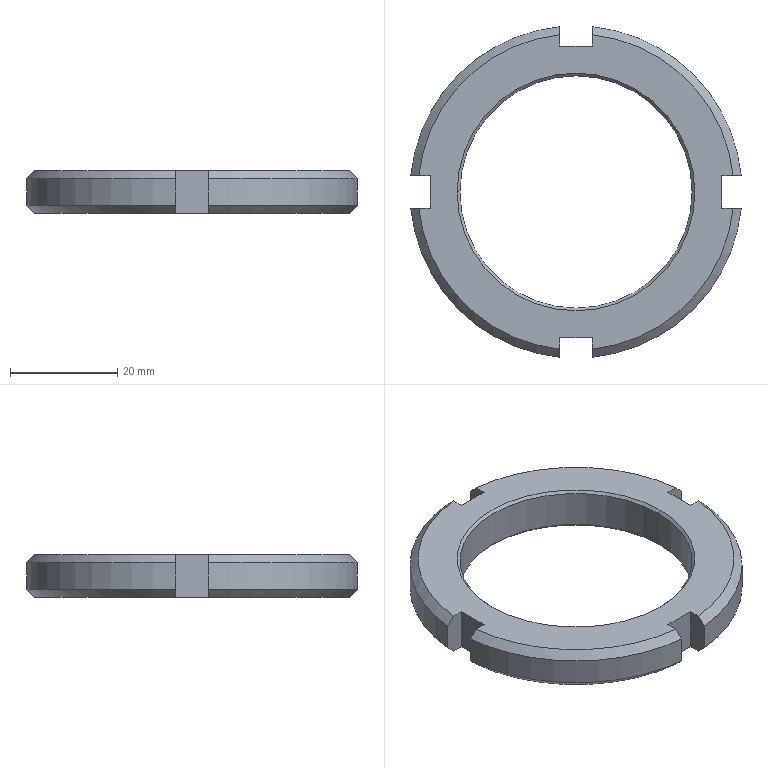Part | SolidWorks | features BaseBody 1 | 1 solid | 32 faces | box 61.709 x 61.709 x 8 mm | volume 11209 mm3 | plane 14 | cone 12 | cylinder 6 | commonest cylinder face diameters 62 x4 43.376 x2
STEP:
#1=CARTESIAN_POINT('',(-21.688,0.,7.5));
#2=VERTEX_POINT('',#1);
#3=CARTESIAN_POINT('',(21.688,0.,7.5));
#4=VERTEX_POINT('',#3);
#5=CARTESIAN_POINT('',(0.,0.,7.5));
#6=DIRECTION('',(0.,0.,1.));
#7=DIRECTION('',(1.,0.,0.));
#8=AXIS2_PLACEMENT_3D('',#5,#6,#7);
#9=CIRCLE('',#8,21.688);
#10=EDGE_CURVE('',#2,#4,#9,.T.);
#11=ORIENTED_EDGE('',*,*,#10,.F.);
#12=CARTESIAN_POINT('',(-22.188,0.,8.));
#13=VERTEX_POINT('',#12);
#14=CARTESIAN_POINT('',(-21.688,0.,7.5));
#15=DIRECTION('',(-0.7071,0.,0.7071));
#16=VECTOR('',#15,1000.);
#17=LINE('',#14,#16);
#18=EDGE_CURVE('',#2,#13,#17,.T.);
#19=ORIENTED_EDGE('',*,*,#18,.T.);
#20=CARTESIAN_POINT('',(22.188,0.,8.));
#21=VERTEX_POINT('',#20);
#22=CARTESIAN_POINT('',(0.,0.,8.));
#23=DIRECTION('',(0.,0.,-1.));
#24=DIRECTION('',(1.,0.,0.));
#25=AXIS2_PLACEMENT_3D('',#22,#23,#24);
#26=CIRCLE('',#25,22.188);
#27=EDGE_CURVE('',#21,#13,#26,.T.);
#28=ORIENTED_EDGE('',*,*,#27,.F.);
#29=CARTESIAN_POINT('',(21.688,0.,7.5));
#30=DIRECTION('',(0.7071,0.,0.7071));
#31=VECTOR('',#30,1000.);
#32=LINE('',#29,#31);
#33=EDGE_CURVE('',#4,#21,#32,.T.);
#34=ORIENTED_EDGE('',*,*,#33,.F.);
#35=EDGE_LOOP('',(#11,#19,#28,#34));
#36=FACE_OUTER_BOUND('',#35,.T.);
#37=CARTESIAN_POINT('',(0.,0.,7.5));
#38=DIRECTION('',(0.,0.,1.));
#39=DIRECTION('',(1.,0.,0.));
#40=AXIS2_PLACEMENT_3D('',#37,#38,#39);
#41=CONICAL_SURFACE('',#40,21.688,0.7854);
#42=ADVANCED_FACE('',(#36),#41,.F.);
#43=CARTESIAN_POINT('',(21.688,0.,0.5));
#44=VERTEX_POINT('',#43);
#45=CARTESIAN_POINT('',(-21.688,0.,0.5));
#46=VERTEX_POINT('',#45);
#47=CARTESIAN_POINT('',(0.,0.,0.5));
#48=DIRECTION('',(0.,0.,-1.));
#49=DIRECTION('',(1.,0.,0.));
#50=AXIS2_PLACEMENT_3D('',#47,#48,#49);
#51=CIRCLE('',#50,21.688);
#52=EDGE_CURVE('',#44,#46,#51,.T.);
#53=ORIENTED_EDGE('',*,*,#52,.F.);
#54=CARTESIAN_POINT('',(22.188,0.,0.));
#55=VERTEX_POINT('',#54);
#56=CARTESIAN_POINT('',(22.188,0.,0.));
#57=DIRECTION('',(0.7071,0.,-0.7071));
#58=VECTOR('',#57,1000.);
#59=LINE('',#56,#58);
#60=EDGE_CURVE('',#44,#55,#59,.T.);
#61=ORIENTED_EDGE('',*,*,#60,.T.);
#62=CARTESIAN_POINT('',(-22.188,0.,0.));
#63=VERTEX_POINT('',#62);
#64=CARTESIAN_POINT('',(0.,0.,0.));
#65=DIRECTION('',(0.,0.,1.));
#66=DIRECTION('',(1.,0.,0.));
#67=AXIS2_PLACEMENT_3D('',#64,#65,#66);
#68=CIRCLE('',#67,22.188);
#69=EDGE_CURVE('',#63,#55,#68,.T.);
#70=ORIENTED_EDGE('',*,*,#69,.F.);
#71=CARTESIAN_POINT('',(-22.188,0.,0.));
#72=DIRECTION('',(-0.7071,0.,-0.7071));
#73=VECTOR('',#72,1000.);
#74=LINE('',#71,#73);
#75=EDGE_CURVE('',#46,#63,#74,.T.);
#76=ORIENTED_EDGE('',*,*,#75,.F.);
#77=EDGE_LOOP('',(#53,#61,#70,#76));
#78=FACE_OUTER_BOUND('',#77,.T.);
#79=CARTESIAN_POINT('',(0.,0.,0.));
#80=DIRECTION('',(0.,0.,-1.));
#81=DIRECTION('',(-1.,0.,0.));
#82=AXIS2_PLACEMENT_3D('',#79,#80,#81);
#83=CONICAL_SURFACE('',#82,22.188,0.7854);
#84=ADVANCED_FACE('',(#78),#83,.F.);
#85=ORIENTED_EDGE('',*,*,#10,.T.);
#86=CARTESIAN_POINT('',(21.688,0.,8.));
#87=DIRECTION('',(0.,0.,-1.));
#88=VECTOR('',#87,1000.);
#89=LINE('',#86,#88);
#90=EDGE_CURVE('',#4,#44,#89,.T.);
#91=ORIENTED_EDGE('',*,*,#90,.T.);
#92=ORIENTED_EDGE('',*,*,#52,.T.);
#93=CARTESIAN_POINT('',(-21.688,0.,8.));
#94=DIRECTION('',(0.,0.,-1.));
#95=VECTOR('',#94,1000.);
#96=LINE('',#93,#95);
#97=EDGE_CURVE('',#2,#46,#96,.T.);
#98=ORIENTED_EDGE('',*,*,#97,.F.);
#99=EDGE_LOOP('',(#85,#91,#92,#98));
#100=FACE_OUTER_BOUND('',#99,.T.);
#101=CARTESIAN_POINT('',(0.,0.,8.));
#102=DIRECTION('',(0.,0.,-1.));
#103=DIRECTION('',(-1.,0.,0.));
#104=AXIS2_PLACEMENT_3D('',#101,#102,#103);
#105=CYLINDRICAL_SURFACE('',#104,21.688);
#106=ADVANCED_FACE('',(#100),#105,.F.);
#107=CARTESIAN_POINT('',(3.,30.854,6.5));
#108=VERTEX_POINT('',#107);
#109=CARTESIAN_POINT('',(30.854,3.,6.5));
#110=VERTEX_POINT('',#109);
#111=CARTESIAN_POINT('',(0.,0.,6.5));
#112=DIRECTION('',(0.,0.,-1.));
#113=DIRECTION('',(1.,0.,0.));
#114=AXIS2_PLACEMENT_3D('',#111,#112,#113);
#115=CIRCLE('',#114,31.);
#116=EDGE_CURVE('',#108,#110,#115,.T.);
#117=ORIENTED_EDGE('',*,*,#116,.T.);
#118=CARTESIAN_POINT('',(30.854,3.,1.5));
#119=VERTEX_POINT('',#118);
#120=CARTESIAN_POINT('',(30.854,3.,0.));
#121=DIRECTION('',(0.,0.,1.));
#122=VECTOR('',#121,1000.);
#123=LINE('',#120,#122);
#124=EDGE_CURVE('',#119,#110,#123,.T.);
#125=ORIENTED_EDGE('',*,*,#124,.F.);
#126=CARTESIAN_POINT('',(3.,30.854,1.5));
#127=VERTEX_POINT('',#126);
#128=CARTESIAN_POINT('',(0.,0.,1.5));
#129=DIRECTION('',(0.,0.,1.));
#130=DIRECTION('',(1.,0.,0.));
#131=AXIS2_PLACEMENT_3D('',#128,#129,#130);
#132=CIRCLE('',#131,31.);
#133=EDGE_CURVE('',#119,#127,#132,.T.);
#134=ORIENTED_EDGE('',*,*,#133,.T.);
#135=CARTESIAN_POINT('',(3.,30.854,0.));
#136=DIRECTION('',(0.,0.,1.));
#137=VECTOR('',#136,1000.);
#138=LINE('',#135,#137);
#139=EDGE_CURVE('',#127,#108,#138,.T.);
#140=ORIENTED_EDGE('',*,*,#139,.T.);
#141=EDGE_LOOP('',(#117,#125,#134,#140));
#142=FACE_OUTER_BOUND('',#141,.T.);
#143=CARTESIAN_POINT('',(0.,0.,8.));
#144=DIRECTION('',(0.,0.,-1.));
#145=DIRECTION('',(-1.,0.,0.));
#146=AXIS2_PLACEMENT_3D('',#143,#144,#145);
#147=CYLINDRICAL_SURFACE('',#146,31.);
#148=ADVANCED_FACE('',(#142),#147,.T.);
#149=CARTESIAN_POINT('',(29.347,3.,8.));
#150=VERTEX_POINT('',#149);
#151=CARTESIAN_POINT('',(30.854,3.,6.5));
#152=CARTESIAN_POINT('',(30.441,3.,6.912));
#153=CARTESIAN_POINT('',(30.027,3.,7.323));
#154=CARTESIAN_POINT('',(29.614,3.,7.735));
#155=CARTESIAN_POINT('',(29.525,3.,7.823));
#156=CARTESIAN_POINT('',(29.436,3.,7.912));
#157=CARTESIAN_POINT('',(29.347,3.,8.));
#158=B_SPLINE_CURVE_WITH_KNOTS('',3,(#151,#152,#153,#154,#155,#156,#157),.UNSPECIFIED.,.F.,.F.,(4,3,4),(0.006071,0.007821,0.008198),.UNSPECIFIED.);
#159=EDGE_CURVE('',#110,#150,#158,.T.);
#160=ORIENTED_EDGE('',*,*,#159,.F.);
#161=ORIENTED_EDGE('',*,*,#116,.F.);
#162=CARTESIAN_POINT('',(3.,29.347,8.));
#163=VERTEX_POINT('',#162);
#164=CARTESIAN_POINT('',(3.,29.347,8.));
#165=CARTESIAN_POINT('',(3.,29.436,7.912));
#166=CARTESIAN_POINT('',(3.,29.525,7.823));
#167=CARTESIAN_POINT('',(3.,29.614,7.735));
#168=CARTESIAN_POINT('',(3.,30.027,7.323));
#169=CARTESIAN_POINT('',(3.,30.441,6.912));
#170=CARTESIAN_POINT('',(3.,30.854,6.5));
#171=B_SPLINE_CURVE_WITH_KNOTS('',3,(#164,#165,#166,#167,#168,#169,#170),.UNSPECIFIED.,.F.,.F.,(4,3,4),(0.007445,0.007821,0.009572),.UNSPECIFIED.);
#172=EDGE_CURVE('',#163,#108,#171,.T.);
#173=ORIENTED_EDGE('',*,*,#172,.F.);
#174=CARTESIAN_POINT('',(0.,0.,8.));
#175=DIRECTION('',(0.,0.,1.));
#176=DIRECTION('',(1.,0.,0.));
#177=AXIS2_PLACEMENT_3D('',#174,#175,#176);
#178=CIRCLE('',#177,29.5);
#179=EDGE_CURVE('',#150,#163,#178,.T.);
#180=ORIENTED_EDGE('',*,*,#179,.F.);
#181=EDGE_LOOP('',(#160,#161,#173,#180));
#182=FACE_OUTER_BOUND('',#181,.T.);
#183=CARTESIAN_POINT('',(0.,0.,8.));
#184=DIRECTION('',(0.,0.,-1.));
#185=DIRECTION('',(-1.,0.,0.));
#186=AXIS2_PLACEMENT_3D('',#183,#184,#185);
#187=CONICAL_SURFACE('',#186,29.5,0.7854);
#188=ADVANCED_FACE('',(#182),#187,.T.);
#189=CARTESIAN_POINT('',(29.347,3.,0.));
#190=VERTEX_POINT('',#189);
#191=CARTESIAN_POINT('',(29.347,3.,0.));
#192=CARTESIAN_POINT('',(29.436,3.,0.08842));
#193=CARTESIAN_POINT('',(29.525,3.,0.1768));
#194=CARTESIAN_POINT('',(29.614,3.,0.2653));
#195=CARTESIAN_POINT('',(30.027,3.,0.6768));
#196=CARTESIAN_POINT('',(30.441,3.,1.088));
#197=CARTESIAN_POINT('',(30.854,3.,1.5));
#198=B_SPLINE_CURVE_WITH_KNOTS('',3,(#191,#192,#193,#194,#195,#196,#197),.UNSPECIFIED.,.F.,.F.,(4,3,4),(0.007445,0.007821,0.009572),.UNSPECIFIED.);
#199=EDGE_CURVE('',#190,#119,#198,.T.);
#200=ORIENTED_EDGE('',*,*,#199,.F.);
#201=CARTESIAN_POINT('',(3.,29.347,0.));
#202=VERTEX_POINT('',#201);
#203=CARTESIAN_POINT('',(0.,0.,0.));
#204=DIRECTION('',(0.,0.,-1.));
#205=DIRECTION('',(1.,0.,0.));
#206=AXIS2_PLACEMENT_3D('',#203,#204,#205);
#207=CIRCLE('',#206,29.5);
#208=EDGE_CURVE('',#202,#190,#207,.T.);
#209=ORIENTED_EDGE('',*,*,#208,.F.);
#210=CARTESIAN_POINT('',(3.,30.854,1.5));
#211=CARTESIAN_POINT('',(3.,30.441,1.088));
#212=CARTESIAN_POINT('',(3.,30.027,0.6768));
#213=CARTESIAN_POINT('',(3.,29.614,0.2653));
#214=CARTESIAN_POINT('',(3.,29.525,0.1768));
#215=CARTESIAN_POINT('',(3.,29.436,0.08842));
#216=CARTESIAN_POINT('',(3.,29.347,0.));
#217=B_SPLINE_CURVE_WITH_KNOTS('',3,(#210,#211,#212,#213,#214,#215,#216),.UNSPECIFIED.,.F.,.F.,(4,3,4),(0.006071,0.007821,0.008198),.UNSPECIFIED.);
#218=EDGE_CURVE('',#127,#202,#217,.T.);
#219=ORIENTED_EDGE('',*,*,#218,.F.);
#220=ORIENTED_EDGE('',*,*,#133,.F.);
#221=EDGE_LOOP('',(#200,#209,#219,#220));
#222=FACE_OUTER_BOUND('',#221,.T.);
#223=CARTESIAN_POINT('',(0.,0.,1.5));
#224=DIRECTION('',(0.,0.,1.));
#225=DIRECTION('',(1.,0.,0.));
#226=AXIS2_PLACEMENT_3D('',#223,#224,#225);
#227=CONICAL_SURFACE('',#226,31.,0.7854);
#228=ADVANCED_FACE('',(#222),#227,.T.);
#229=CARTESIAN_POINT('',(-30.854,3.,6.5));
#230=VERTEX_POINT('',#229);
#231=CARTESIAN_POINT('',(-3.,30.854,6.5));
#232=VERTEX_POINT('',#231);
#233=CARTESIAN_POINT('',(0.,0.,6.5));
#234=DIRECTION('',(0.,0.,-1.));
#235=DIRECTION('',(1.,0.,0.));
#236=AXIS2_PLACEMENT_3D('',#233,#234,#235);
#237=CIRCLE('',#236,31.);
#238=EDGE_CURVE('',#230,#232,#237,.T.);
#239=ORIENTED_EDGE('',*,*,#238,.T.);
#240=CARTESIAN_POINT('',(-3.,30.854,1.5));
#241=VERTEX_POINT('',#240);
#242=CARTESIAN_POINT('',(-3.,30.854,0.));
#243=DIRECTION('',(0.,0.,1.));
#244=VECTOR('',#243,1000.);
#245=LINE('',#242,#244);
#246=EDGE_CURVE('',#241,#232,#245,.T.);
#247=ORIENTED_EDGE('',*,*,#246,.F.);
#248=CARTESIAN_POINT('',(-30.854,3.,1.5));
#249=VERTEX_POINT('',#248);
#250=CARTESIAN_POINT('',(0.,0.,1.5));
#251=DIRECTION('',(0.,0.,1.));
#252=DIRECTION('',(1.,0.,0.));
#253=AXIS2_PLACEMENT_3D('',#250,#251,#252);
#254=CIRCLE('',#253,31.);
#255=EDGE_CURVE('',#241,#249,#254,.T.);
#256=ORIENTED_EDGE('',*,*,#255,.T.);
#257=CARTESIAN_POINT('',(-30.854,3.,0.));
#258=DIRECTION('',(0.,0.,1.));
#259=VECTOR('',#258,1000.);
#260=LINE('',#257,#259);
#261=EDGE_CURVE('',#249,#230,#260,.T.);
#262=ORIENTED_EDGE('',*,*,#261,.T.);
#263=EDGE_LOOP('',(#239,#247,#256,#262));
#264=FACE_OUTER_BOUND('',#263,.T.);
#265=CARTESIAN_POINT('',(0.,0.,8.));
#266=DIRECTION('',(0.,0.,-1.));
#267=DIRECTION('',(-1.,0.,0.));
#268=AXIS2_PLACEMENT_3D('',#265,#266,#267);
#269=CYLINDRICAL_SURFACE('',#268,31.);
#270=ADVANCED_FACE('',(#264),#269,.T.);
#271=CARTESIAN_POINT('',(-3.,29.347,8.));
#272=VERTEX_POINT('',#271);
#273=CARTESIAN_POINT('',(-3.,30.854,6.5));
#274=CARTESIAN_POINT('',(-3.,30.441,6.912));
#275=CARTESIAN_POINT('',(-3.,30.027,7.323));
#276=CARTESIAN_POINT('',(-3.,29.614,7.735));
#277=CARTESIAN_POINT('',(-3.,29.525,7.823));
#278=CARTESIAN_POINT('',(-3.,29.436,7.912));
#279=CARTESIAN_POINT('',(-3.,29.347,8.));
#280=B_SPLINE_CURVE_WITH_KNOTS('',3,(#273,#274,#275,#276,#277,#278,#279),.UNSPECIFIED.,.F.,.F.,(4,3,4),(0.006071,0.007821,0.008198),.UNSPECIFIED.);
#281=EDGE_CURVE('',#232,#272,#280,.T.);
#282=ORIENTED_EDGE('',*,*,#281,.F.);
#283=ORIENTED_EDGE('',*,*,#238,.F.);
#284=CARTESIAN_POINT('',(-29.347,3.,8.));
#285=VERTEX_POINT('',#284);
#286=CARTESIAN_POINT('',(-29.347,3.,8.));
#287=CARTESIAN_POINT('',(-29.712,3.,7.637));
#288=CARTESIAN_POINT('',(-30.076,3.,7.274));
#289=CARTESIAN_POINT('',(-30.441,3.,6.912));
#290=CARTESIAN_POINT('',(-30.579,3.,6.774));
#291=CARTESIAN_POINT('',(-30.717,3.,6.637));
#292=CARTESIAN_POINT('',(-30.854,3.,6.5));
#293=B_SPLINE_CURVE_WITH_KNOTS('',3,(#286,#287,#288,#289,#290,#291,#292),.UNSPECIFIED.,.F.,.F.,(4,3,4),(0.006278,0.007821,0.008405),.UNSPECIFIED.);
#294=EDGE_CURVE('',#285,#230,#293,.T.);
#295=ORIENTED_EDGE('',*,*,#294,.F.);
#296=CARTESIAN_POINT('',(0.,0.,8.));
#297=DIRECTION('',(0.,0.,1.));
#298=DIRECTION('',(1.,0.,0.));
#299=AXIS2_PLACEMENT_3D('',#296,#297,#298);
#300=CIRCLE('',#299,29.5);
#301=EDGE_CURVE('',#272,#285,#300,.T.);
#302=ORIENTED_EDGE('',*,*,#301,.F.);
#303=EDGE_LOOP('',(#282,#283,#295,#302));
#304=FACE_OUTER_BOUND('',#303,.T.);
#305=CARTESIAN_POINT('',(0.,0.,8.));
#306=DIRECTION('',(0.,0.,-1.));
#307=DIRECTION('',(-1.,0.,0.));
#308=AXIS2_PLACEMENT_3D('',#305,#306,#307);
#309=CONICAL_SURFACE('',#308,29.5,0.7854);
#310=ADVANCED_FACE('',(#304),#309,.T.);
#311=CARTESIAN_POINT('',(-3.,29.347,0.));
#312=VERTEX_POINT('',#311);
#313=CARTESIAN_POINT('',(-3.,29.347,0.));
#314=CARTESIAN_POINT('',(-3.,29.436,0.08842));
#315=CARTESIAN_POINT('',(-3.,29.525,0.1768));
#316=CARTESIAN_POINT('',(-3.,29.614,0.2653));
#317=CARTESIAN_POINT('',(-3.,30.027,0.6768));
#318=CARTESIAN_POINT('',(-3.,30.441,1.088));
#319=CARTESIAN_POINT('',(-3.,30.854,1.5));
#320=B_SPLINE_CURVE_WITH_KNOTS('',3,(#313,#314,#315,#316,#317,#318,#319),.UNSPECIFIED.,.F.,.F.,(4,3,4),(0.007445,0.007821,0.009572),.UNSPECIFIED.);
#321=EDGE_CURVE('',#312,#241,#320,.T.);
#322=ORIENTED_EDGE('',*,*,#321,.F.);
#323=CARTESIAN_POINT('',(-29.347,3.,0.));
#324=VERTEX_POINT('',#323);
#325=CARTESIAN_POINT('',(0.,0.,0.));
#326=DIRECTION('',(0.,0.,-1.));
#327=DIRECTION('',(1.,0.,0.));
#328=AXIS2_PLACEMENT_3D('',#325,#326,#327);
#329=CIRCLE('',#328,29.5);
#330=EDGE_CURVE('',#324,#312,#329,.T.);
#331=ORIENTED_EDGE('',*,*,#330,.F.);
#332=CARTESIAN_POINT('',(-30.854,3.,1.5));
#333=CARTESIAN_POINT('',(-30.592,3.,1.238));
#334=CARTESIAN_POINT('',(-30.329,3.,0.9768));
#335=CARTESIAN_POINT('',(-30.066,3.,0.7152));
#336=CARTESIAN_POINT('',(-29.826,3.,0.4768));
#337=CARTESIAN_POINT('',(-29.587,3.,0.2384));
#338=CARTESIAN_POINT('',(-29.347,3.,0.));
#339=B_SPLINE_CURVE_WITH_KNOTS('',3,(#332,#333,#334,#335,#336,#337,#338),.UNSPECIFIED.,.F.,.F.,(4,3,4),(0.006709,0.007821,0.008836),.UNSPECIFIED.);
#340=EDGE_CURVE('',#249,#324,#339,.T.);
#341=ORIENTED_EDGE('',*,*,#340,.F.);
#342=ORIENTED_EDGE('',*,*,#255,.F.);
#343=EDGE_LOOP('',(#322,#331,#341,#342));
#344=FACE_OUTER_BOUND('',#343,.T.);
#345=CARTESIAN_POINT('',(0.,0.,1.5));
#346=DIRECTION('',(0.,0.,1.));
#347=DIRECTION('',(1.,0.,0.));
#348=AXIS2_PLACEMENT_3D('',#345,#346,#347);
#349=CONICAL_SURFACE('',#348,31.,0.7854);
#350=ADVANCED_FACE('',(#344),#349,.T.);
#351=CARTESIAN_POINT('',(-3.,-30.854,6.5));
#352=VERTEX_POINT('',#351);
#353=CARTESIAN_POINT('',(-30.854,-3.,6.5));
#354=VERTEX_POINT('',#353);
#355=CARTESIAN_POINT('',(0.,0.,6.5));
#356=DIRECTION('',(0.,0.,-1.));
#357=DIRECTION('',(1.,0.,0.));
#358=AXIS2_PLACEMENT_3D('',#355,#356,#357);
#359=CIRCLE('',#358,31.);
#360=EDGE_CURVE('',#352,#354,#359,.T.);
#361=ORIENTED_EDGE('',*,*,#360,.T.);
#362=CARTESIAN_POINT('',(-30.854,-3.,1.5));
#363=VERTEX_POINT('',#362);
#364=CARTESIAN_POINT('',(-30.854,-3.,0.));
#365=DIRECTION('',(0.,0.,1.));
#366=VECTOR('',#365,1000.);
#367=LINE('',#364,#366);
#368=EDGE_CURVE('',#363,#354,#367,.T.);
#369=ORIENTED_EDGE('',*,*,#368,.F.);
#370=CARTESIAN_POINT('',(-3.,-30.854,1.5));
#371=VERTEX_POINT('',#370);
#372=CARTESIAN_POINT('',(0.,0.,1.5));
#373=DIRECTION('',(0.,0.,1.));
#374=DIRECTION('',(1.,0.,0.));
#375=AXIS2_PLACEMENT_3D('',#372,#373,#374);
#376=CIRCLE('',#375,31.);
#377=EDGE_CURVE('',#363,#371,#376,.T.);
#378=ORIENTED_EDGE('',*,*,#377,.T.);
#379=CARTESIAN_POINT('',(-3.,-30.854,0.));
#380=DIRECTION('',(0.,0.,1.));
#381=VECTOR('',#380,1000.);
#382=LINE('',#379,#381);
#383=EDGE_CURVE('',#371,#352,#382,.T.);
#384=ORIENTED_EDGE('',*,*,#383,.T.);
#385=EDGE_LOOP('',(#361,#369,#378,#384));
#386=FACE_OUTER_BOUND('',#385,.T.);
#387=CARTESIAN_POINT('',(0.,0.,8.));
#388=DIRECTION('',(0.,0.,-1.));
#389=DIRECTION('',(-1.,0.,0.));
#390=AXIS2_PLACEMENT_3D('',#387,#388,#389);
#391=CYLINDRICAL_SURFACE('',#390,31.);
#392=ADVANCED_FACE('',(#386),#391,.T.);
#393=CARTESIAN_POINT('',(-29.347,-3.,8.));
#394=VERTEX_POINT('',#393);
#395=CARTESIAN_POINT('',(-30.854,-3.,6.5));
#396=CARTESIAN_POINT('',(-30.717,-3.,6.637));
#397=CARTESIAN_POINT('',(-30.579,-3.,6.774));
#398=CARTESIAN_POINT('',(-30.441,-3.,6.912));
#399=CARTESIAN_POINT('',(-30.076,-3.,7.274));
#400=CARTESIAN_POINT('',(-29.712,-3.,7.637));
#401=CARTESIAN_POINT('',(-29.347,-3.,8.));
#402=B_SPLINE_CURVE_WITH_KNOTS('',3,(#395,#396,#397,#398,#399,#400,#401),.UNSPECIFIED.,.F.,.F.,(4,3,4),(0.007238,0.007821,0.009365),.UNSPECIFIED.);
#403=EDGE_CURVE('',#354,#394,#402,.T.);
#404=ORIENTED_EDGE('',*,*,#403,.F.);
#405=ORIENTED_EDGE('',*,*,#360,.F.);
#406=CARTESIAN_POINT('',(-3.,-29.347,8.));
#407=VERTEX_POINT('',#406);
#408=CARTESIAN_POINT('',(-3.,-29.347,8.));
#409=CARTESIAN_POINT('',(-3.,-29.85,7.5));
#410=CARTESIAN_POINT('',(-3.,-30.352,7.));
#411=CARTESIAN_POINT('',(-3.,-30.854,6.5));
#412=B_SPLINE_CURVE_WITH_KNOTS('',3,(#408,#409,#410,#411),.UNSPECIFIED.,.F.,.F.,(4,4),(0.,0.002127),.UNSPECIFIED.);
#413=EDGE_CURVE('',#407,#352,#412,.T.);
#414=ORIENTED_EDGE('',*,*,#413,.F.);
#415=CARTESIAN_POINT('',(0.,0.,8.));
#416=DIRECTION('',(0.,0.,1.));
#417=DIRECTION('',(1.,0.,0.));
#418=AXIS2_PLACEMENT_3D('',#415,#416,#417);
#419=CIRCLE('',#418,29.5);
#420=EDGE_CURVE('',#394,#407,#419,.T.);
#421=ORIENTED_EDGE('',*,*,#420,.F.);
#422=EDGE_LOOP('',(#404,#405,#414,#421));
#423=FACE_OUTER_BOUND('',#422,.T.);
#424=CARTESIAN_POINT('',(0.,0.,8.));
#425=DIRECTION('',(0.,0.,-1.));
#426=DIRECTION('',(-1.,0.,0.));
#427=AXIS2_PLACEMENT_3D('',#424,#425,#426);
#428=CONICAL_SURFACE('',#427,29.5,0.7854);
#429=ADVANCED_FACE('',(#423),#428,.T.);
#430=CARTESIAN_POINT('',(-29.347,-3.,0.));
#431=VERTEX_POINT('',#430);
#432=CARTESIAN_POINT('',(-29.347,-3.,0.));
#433=CARTESIAN_POINT('',(-29.587,-3.,0.2384));
#434=CARTESIAN_POINT('',(-29.826,-3.,0.4768));
#435=CARTESIAN_POINT('',(-30.066,-3.,0.7152));
#436=CARTESIAN_POINT('',(-30.329,-3.,0.9768));
#437=CARTESIAN_POINT('',(-30.592,-3.,1.238));
#438=CARTESIAN_POINT('',(-30.854,-3.,1.5));
#439=B_SPLINE_CURVE_WITH_KNOTS('',3,(#432,#433,#434,#435,#436,#437,#438),.UNSPECIFIED.,.F.,.F.,(4,3,4),(0.006807,0.007821,0.008934),.UNSPECIFIED.);
#440=EDGE_CURVE('',#431,#363,#439,.T.);
#441=ORIENTED_EDGE('',*,*,#440,.F.);
#442=CARTESIAN_POINT('',(-3.,-29.347,0.));
#443=VERTEX_POINT('',#442);
#444=CARTESIAN_POINT('',(0.,0.,0.));
#445=DIRECTION('',(0.,0.,-1.));
#446=DIRECTION('',(1.,0.,0.));
#447=AXIS2_PLACEMENT_3D('',#444,#445,#446);
#448=CIRCLE('',#447,29.5);
#449=EDGE_CURVE('',#443,#431,#448,.T.);
#450=ORIENTED_EDGE('',*,*,#449,.F.);
#451=CARTESIAN_POINT('',(-3.,-30.854,1.5));
#452=CARTESIAN_POINT('',(-3.,-30.352,0.9999));
#453=CARTESIAN_POINT('',(-3.,-29.85,0.4999));
#454=CARTESIAN_POINT('',(-3.,-29.347,0.));
#455=B_SPLINE_CURVE_WITH_KNOTS('',3,(#451,#452,#453,#454),.UNSPECIFIED.,.F.,.F.,(4,4),(0.,0.002127),.UNSPECIFIED.);
#456=EDGE_CURVE('',#371,#443,#455,.T.);
#457=ORIENTED_EDGE('',*,*,#456,.F.);
#458=ORIENTED_EDGE('',*,*,#377,.F.);
#459=EDGE_LOOP('',(#441,#450,#457,#458));
#460=FACE_OUTER_BOUND('',#459,.T.);
#461=CARTESIAN_POINT('',(0.,0.,1.5));
#462=DIRECTION('',(0.,0.,1.));
#463=DIRECTION('',(1.,0.,0.));
#464=AXIS2_PLACEMENT_3D('',#461,#462,#463);
#465=CONICAL_SURFACE('',#464,31.,0.7854);
#466=ADVANCED_FACE('',(#460),#465,.T.);
#467=ORIENTED_EDGE('',*,*,#27,.T.);
#468=CARTESIAN_POINT('',(0.,0.,8.));
#469=DIRECTION('',(0.,0.,-1.));
#470=DIRECTION('',(1.,0.,0.));
#471=AXIS2_PLACEMENT_3D('',#468,#469,#470);
#472=CIRCLE('',#471,22.188);
#473=EDGE_CURVE('',#13,#21,#472,.T.);
#474=ORIENTED_EDGE('',*,*,#473,.T.);
#475=EDGE_LOOP('',(#467,#474));
#476=FACE_BOUND('',#475,.T.);
#477=CARTESIAN_POINT('',(27.254,3.,8.));
#478=VERTEX_POINT('',#477);
#479=CARTESIAN_POINT('',(27.254,3.,8.));
#480=DIRECTION('',(-1.,0.,0.));
#481=VECTOR('',#480,1000.);
#482=LINE('',#479,#481);
#483=EDGE_CURVE('',#150,#478,#482,.T.);
#484=ORIENTED_EDGE('',*,*,#483,.F.);
#485=ORIENTED_EDGE('',*,*,#179,.T.);
#486=CARTESIAN_POINT('',(3.,27.254,8.));
#487=VERTEX_POINT('',#486);
#488=CARTESIAN_POINT('',(3.,27.254,8.));
#489=DIRECTION('',(0.,1.,0.));
#490=VECTOR('',#489,1000.);
#491=LINE('',#488,#490);
#492=EDGE_CURVE('',#487,#163,#491,.T.);
#493=ORIENTED_EDGE('',*,*,#492,.F.);
#494=CARTESIAN_POINT('',(-3.,27.254,8.));
#495=VERTEX_POINT('',#494);
#496=CARTESIAN_POINT('',(3.,27.254,8.));
#497=DIRECTION('',(1.,0.,0.));
#498=VECTOR('',#497,1000.);
#499=LINE('',#496,#498);
#500=EDGE_CURVE('',#495,#487,#499,.T.);
#501=ORIENTED_EDGE('',*,*,#500,.F.);
#502=CARTESIAN_POINT('',(-3.,27.254,8.));
#503=DIRECTION('',(0.,-1.,0.));
#504=VECTOR('',#503,1000.);
#505=LINE('',#502,#504);
#506=EDGE_CURVE('',#272,#495,#505,.T.);
#507=ORIENTED_EDGE('',*,*,#506,.F.);
#508=ORIENTED_EDGE('',*,*,#301,.T.);
#509=CARTESIAN_POINT('',(-27.254,3.,8.));
#510=VERTEX_POINT('',#509);
#511=CARTESIAN_POINT('',(-27.254,3.,8.));
#512=DIRECTION('',(-1.,0.,0.));
#513=VECTOR('',#512,1000.);
#514=LINE('',#511,#513);
#515=EDGE_CURVE('',#510,#285,#514,.T.);
#516=ORIENTED_EDGE('',*,*,#515,.F.);
#517=CARTESIAN_POINT('',(-27.254,-3.,8.));
#518=VERTEX_POINT('',#517);
#519=CARTESIAN_POINT('',(-27.254,3.,8.));
#520=DIRECTION('',(0.,1.,0.));
#521=VECTOR('',#520,1000.);
#522=LINE('',#519,#521);
#523=EDGE_CURVE('',#518,#510,#522,.T.);
#524=ORIENTED_EDGE('',*,*,#523,.F.);
#525=CARTESIAN_POINT('',(-27.254,-3.,8.));
#526=DIRECTION('',(1.,0.,0.));
#527=VECTOR('',#526,1000.);
#528=LINE('',#525,#527);
#529=EDGE_CURVE('',#394,#518,#528,.T.);
#530=ORIENTED_EDGE('',*,*,#529,.F.);
#531=ORIENTED_EDGE('',*,*,#420,.T.);
#532=CARTESIAN_POINT('',(-3.,-27.254,8.));
#533=VERTEX_POINT('',#532);
#534=CARTESIAN_POINT('',(-3.,-27.254,8.));
#535=DIRECTION('',(0.,-1.,0.));
#536=VECTOR('',#535,1000.);
#537=LINE('',#534,#536);
#538=EDGE_CURVE('',#533,#407,#537,.T.);
#539=ORIENTED_EDGE('',*,*,#538,.F.);
#540=CARTESIAN_POINT('',(3.,-27.254,8.));
#541=VERTEX_POINT('',#540);
#542=CARTESIAN_POINT('',(-3.,-27.254,8.));
#543=DIRECTION('',(-1.,0.,0.));
#544=VECTOR('',#543,1000.);
#545=LINE('',#542,#544);
#546=EDGE_CURVE('',#541,#533,#545,.T.);
#547=ORIENTED_EDGE('',*,*,#546,.F.);
#548=CARTESIAN_POINT('',(3.,-29.347,8.));
#549=VERTEX_POINT('',#548);
#550=CARTESIAN_POINT('',(3.,-27.254,8.));
#551=DIRECTION('',(0.,1.,0.));
#552=VECTOR('',#551,1000.);
#553=LINE('',#550,#552);
#554=EDGE_CURVE('',#549,#541,#553,.T.);
#555=ORIENTED_EDGE('',*,*,#554,.F.);
#556=CARTESIAN_POINT('',(29.347,-3.,8.));
#557=VERTEX_POINT('',#556);
#558=CARTESIAN_POINT('',(0.,0.,8.));
#559=DIRECTION('',(0.,0.,1.));
#560=DIRECTION('',(1.,0.,0.));
#561=AXIS2_PLACEMENT_3D('',#558,#559,#560);
#562=CIRCLE('',#561,29.5);
#563=EDGE_CURVE('',#549,#557,#562,.T.);
#564=ORIENTED_EDGE('',*,*,#563,.T.);
#565=CARTESIAN_POINT('',(27.254,-3.,8.));
#566=VERTEX_POINT('',#565);
#567=CARTESIAN_POINT('',(27.254,-3.,8.));
#568=DIRECTION('',(1.,0.,0.));
#569=VECTOR('',#568,1000.);
#570=LINE('',#567,#569);
#571=EDGE_CURVE('',#566,#557,#570,.T.);
#572=ORIENTED_EDGE('',*,*,#571,.F.);
#573=CARTESIAN_POINT('',(27.254,-3.,8.));
#574=DIRECTION('',(0.,-1.,0.));
#575=VECTOR('',#574,1000.);
#576=LINE('',#573,#575);
#577=EDGE_CURVE('',#478,#566,#576,.T.);
#578=ORIENTED_EDGE('',*,*,#577,.F.);
#579=EDGE_LOOP('',(#484,#485,#493,#501,#507,#508,#516,#524,#530,#531,#539,#547,#555,#564,#572,#578));
#580=FACE_OUTER_BOUND('',#579,.T.);
#581=CARTESIAN_POINT('',(0.,0.,8.));
#582=DIRECTION('',(0.,0.,1.));
#583=DIRECTION('',(1.,0.,0.));
#584=AXIS2_PLACEMENT_3D('',#581,#582,#583);
#585=PLANE('',#584);
#586=ADVANCED_FACE('',(#476,#580),#585,.T.);
#587=ORIENTED_EDGE('',*,*,#69,.T.);
#588=CARTESIAN_POINT('',(0.,0.,0.));
#589=DIRECTION('',(0.,0.,1.));
#590=DIRECTION('',(1.,0.,0.));
#591=AXIS2_PLACEMENT_3D('',#588,#589,#590);
#592=CIRCLE('',#591,22.188);
#593=EDGE_CURVE('',#55,#63,#592,.T.);
#594=ORIENTED_EDGE('',*,*,#593,.T.);
#595=EDGE_LOOP('',(#587,#594));
#596=FACE_BOUND('',#595,.T.);
#597=ORIENTED_EDGE('',*,*,#208,.T.);
#598=CARTESIAN_POINT('',(27.254,3.,0.));
#599=VERTEX_POINT('',#598);
#600=CARTESIAN_POINT('',(27.254,3.,0.));
#601=DIRECTION('',(-1.,0.,0.));
#602=VECTOR('',#601,1000.);
#603=LINE('',#600,#602);
#604=EDGE_CURVE('',#190,#599,#603,.T.);
#605=ORIENTED_EDGE('',*,*,#604,.T.);
#606=CARTESIAN_POINT('',(27.254,-3.,0.));
#607=VERTEX_POINT('',#606);
#608=CARTESIAN_POINT('',(27.254,-3.,0.));
#609=DIRECTION('',(0.,-1.,0.));
#610=VECTOR('',#609,1000.);
#611=LINE('',#608,#610);
#612=EDGE_CURVE('',#599,#607,#611,.T.);
#613=ORIENTED_EDGE('',*,*,#612,.T.);
#614=CARTESIAN_POINT('',(29.347,-3.,0.));
#615=VERTEX_POINT('',#614);
#616=CARTESIAN_POINT('',(27.254,-3.,0.));
#617=DIRECTION('',(1.,0.,0.));
#618=VECTOR('',#617,1000.);
#619=LINE('',#616,#618);
#620=EDGE_CURVE('',#607,#615,#619,.T.);
#621=ORIENTED_EDGE('',*,*,#620,.T.);
#622=CARTESIAN_POINT('',(3.,-29.347,0.));
#623=VERTEX_POINT('',#622);
#624=CARTESIAN_POINT('',(0.,0.,0.));
#625=DIRECTION('',(0.,0.,-1.));
#626=DIRECTION('',(1.,0.,0.));
#627=AXIS2_PLACEMENT_3D('',#624,#625,#626);
#628=CIRCLE('',#627,29.5);
#629=EDGE_CURVE('',#615,#623,#628,.T.);
#630=ORIENTED_EDGE('',*,*,#629,.T.);
#631=CARTESIAN_POINT('',(3.,-27.254,0.));
#632=VERTEX_POINT('',#631);
#633=CARTESIAN_POINT('',(3.,-27.254,0.));
#634=DIRECTION('',(0.,1.,0.));
#635=VECTOR('',#634,1000.);
#636=LINE('',#633,#635);
#637=EDGE_CURVE('',#623,#632,#636,.T.);
#638=ORIENTED_EDGE('',*,*,#637,.T.);
#639=CARTESIAN_POINT('',(-3.,-27.254,0.));
#640=VERTEX_POINT('',#639);
#641=CARTESIAN_POINT('',(-3.,-27.254,0.));
#642=DIRECTION('',(-1.,0.,0.));
#643=VECTOR('',#642,1000.);
#644=LINE('',#641,#643);
#645=EDGE_CURVE('',#632,#640,#644,.T.);
#646=ORIENTED_EDGE('',*,*,#645,.T.);
#647=CARTESIAN_POINT('',(-3.,-27.254,0.));
#648=DIRECTION('',(0.,-1.,0.));
#649=VECTOR('',#648,1000.);
#650=LINE('',#647,#649);
#651=EDGE_CURVE('',#640,#443,#650,.T.);
#652=ORIENTED_EDGE('',*,*,#651,.T.);
#653=ORIENTED_EDGE('',*,*,#449,.T.);
#654=CARTESIAN_POINT('',(-27.254,-3.,0.));
#655=VERTEX_POINT('',#654);
#656=CARTESIAN_POINT('',(-27.254,-3.,0.));
#657=DIRECTION('',(1.,0.,0.));
#658=VECTOR('',#657,1000.);
#659=LINE('',#656,#658);
#660=EDGE_CURVE('',#431,#655,#659,.T.);
#661=ORIENTED_EDGE('',*,*,#660,.T.);
#662=CARTESIAN_POINT('',(-27.254,3.,0.));
#663=VERTEX_POINT('',#662);
#664=CARTESIAN_POINT('',(-27.254,3.,0.));
#665=DIRECTION('',(0.,1.,0.));
#666=VECTOR('',#665,1000.);
#667=LINE('',#664,#666);
#668=EDGE_CURVE('',#655,#663,#667,.T.);
#669=ORIENTED_EDGE('',*,*,#668,.T.);
#670=CARTESIAN_POINT('',(-27.254,3.,0.));
#671=DIRECTION('',(-1.,0.,0.));
#672=VECTOR('',#671,1000.);
#673=LINE('',#670,#672);
#674=EDGE_CURVE('',#663,#324,#673,.T.);
#675=ORIENTED_EDGE('',*,*,#674,.T.);
#676=ORIENTED_EDGE('',*,*,#330,.T.);
#677=CARTESIAN_POINT('',(-3.,27.254,0.));
#678=VERTEX_POINT('',#677);
#679=CARTESIAN_POINT('',(-3.,27.254,0.));
#680=DIRECTION('',(0.,-1.,0.));
#681=VECTOR('',#680,1000.);
#682=LINE('',#679,#681);
#683=EDGE_CURVE('',#312,#678,#682,.T.);
#684=ORIENTED_EDGE('',*,*,#683,.T.);
#685=CARTESIAN_POINT('',(3.,27.254,0.));
#686=VERTEX_POINT('',#685);
#687=CARTESIAN_POINT('',(3.,27.254,0.));
#688=DIRECTION('',(1.,0.,0.));
#689=VECTOR('',#688,1000.);
#690=LINE('',#687,#689);
#691=EDGE_CURVE('',#678,#686,#690,.T.);
#692=ORIENTED_EDGE('',*,*,#691,.T.);
#693=CARTESIAN_POINT('',(3.,27.254,0.));
#694=DIRECTION('',(0.,1.,0.));
#695=VECTOR('',#694,1000.);
#696=LINE('',#693,#695);
#697=EDGE_CURVE('',#686,#202,#696,.T.);
#698=ORIENTED_EDGE('',*,*,#697,.T.);
#699=EDGE_LOOP('',(#597,#605,#613,#621,#630,#638,#646,#652,#653,#661,#669,#675,#676,#684,#692,#698));
#700=FACE_OUTER_BOUND('',#699,.T.);
#701=CARTESIAN_POINT('',(0.,0.,0.));
#702=DIRECTION('',(0.,0.,1.));
#703=DIRECTION('',(1.,0.,0.));
#704=AXIS2_PLACEMENT_3D('',#701,#702,#703);
#705=PLANE('',#704);
#706=ADVANCED_FACE('',(#596,#700),#705,.F.);
#707=CARTESIAN_POINT('',(3.,-30.854,1.5));
#708=VERTEX_POINT('',#707);
#709=CARTESIAN_POINT('',(30.854,-3.,1.5));
#710=VERTEX_POINT('',#709);
#711=CARTESIAN_POINT('',(0.,0.,1.5));
#712=DIRECTION('',(0.,0.,1.));
#713=DIRECTION('',(1.,0.,0.));
#714=AXIS2_PLACEMENT_3D('',#711,#712,#713);
#715=CIRCLE('',#714,31.);
#716=EDGE_CURVE('',#708,#710,#715,.T.);
#717=ORIENTED_EDGE('',*,*,#716,.T.);
#718=CARTESIAN_POINT('',(30.854,-3.,6.5));
#719=VERTEX_POINT('',#718);
#720=CARTESIAN_POINT('',(30.854,-3.,0.));
#721=DIRECTION('',(0.,0.,1.));
#722=VECTOR('',#721,1000.);
#723=LINE('',#720,#722);
#724=EDGE_CURVE('',#710,#719,#723,.T.);
#725=ORIENTED_EDGE('',*,*,#724,.T.);
#726=CARTESIAN_POINT('',(3.,-30.854,6.5));
#727=VERTEX_POINT('',#726);
#728=CARTESIAN_POINT('',(0.,0.,6.5));
#729=DIRECTION('',(0.,0.,-1.));
#730=DIRECTION('',(1.,0.,0.));
#731=AXIS2_PLACEMENT_3D('',#728,#729,#730);
#732=CIRCLE('',#731,31.);
#733=EDGE_CURVE('',#719,#727,#732,.T.);
#734=ORIENTED_EDGE('',*,*,#733,.T.);
#735=CARTESIAN_POINT('',(3.,-30.854,0.));
#736=DIRECTION('',(0.,0.,1.));
#737=VECTOR('',#736,1000.);
#738=LINE('',#735,#737);
#739=EDGE_CURVE('',#708,#727,#738,.T.);
#740=ORIENTED_EDGE('',*,*,#739,.F.);
#741=EDGE_LOOP('',(#717,#725,#734,#740));
#742=FACE_OUTER_BOUND('',#741,.T.);
#743=CARTESIAN_POINT('',(0.,0.,8.));
#744=DIRECTION('',(0.,0.,-1.));
#745=DIRECTION('',(-1.,0.,0.));
#746=AXIS2_PLACEMENT_3D('',#743,#744,#745);
#747=CYLINDRICAL_SURFACE('',#746,31.);
#748=ADVANCED_FACE('',(#742),#747,.T.);
#749=ORIENTED_EDGE('',*,*,#90,.F.);
#750=CARTESIAN_POINT('',(0.,0.,7.5));
#751=DIRECTION('',(0.,0.,1.));
#752=DIRECTION('',(1.,0.,0.));
#753=AXIS2_PLACEMENT_3D('',#750,#751,#752);
#754=CIRCLE('',#753,21.688);
#755=EDGE_CURVE('',#4,#2,#754,.T.);
#756=ORIENTED_EDGE('',*,*,#755,.T.);
#757=ORIENTED_EDGE('',*,*,#97,.T.);
#758=CARTESIAN_POINT('',(0.,0.,0.5));
#759=DIRECTION('',(0.,0.,-1.));
#760=DIRECTION('',(1.,0.,0.));
#761=AXIS2_PLACEMENT_3D('',#758,#759,#760);
#762=CIRCLE('',#761,21.688);
#763=EDGE_CURVE('',#46,#44,#762,.T.);
#764=ORIENTED_EDGE('',*,*,#763,.T.);
#765=EDGE_LOOP('',(#749,#756,#757,#764));
#766=FACE_OUTER_BOUND('',#765,.T.);
#767=CARTESIAN_POINT('',(0.,0.,8.));
#768=DIRECTION('',(0.,0.,-1.));
#769=DIRECTION('',(-1.,0.,0.));
#770=AXIS2_PLACEMENT_3D('',#767,#768,#769);
#771=CYLINDRICAL_SURFACE('',#770,21.688);
#772=ADVANCED_FACE('',(#766),#771,.F.);
#773=ORIENTED_EDGE('',*,*,#546,.T.);
#774=CARTESIAN_POINT('',(-3.,-27.254,0.));
#775=DIRECTION('',(0.,0.,1.));
#776=VECTOR('',#775,1000.);
#777=LINE('',#774,#776);
#778=EDGE_CURVE('',#640,#533,#777,.T.);
#779=ORIENTED_EDGE('',*,*,#778,.F.);
#780=ORIENTED_EDGE('',*,*,#645,.F.);
#781=CARTESIAN_POINT('',(3.,-27.254,0.));
#782=DIRECTION('',(0.,0.,1.));
#783=VECTOR('',#782,1000.);
#784=LINE('',#781,#783);
#785=EDGE_CURVE('',#632,#541,#784,.T.);
#786=ORIENTED_EDGE('',*,*,#785,.T.);
#787=EDGE_LOOP('',(#773,#779,#780,#786));
#788=FACE_OUTER_BOUND('',#787,.T.);
#789=CARTESIAN_POINT('',(-3.,-27.254,0.));
#790=DIRECTION('',(0.,1.,0.));
#791=DIRECTION('',(0.,0.,1.));
#792=AXIS2_PLACEMENT_3D('',#789,#790,#791);
#793=PLANE('',#792);
#794=ADVANCED_FACE('',(#788),#793,.F.);
#795=ORIENTED_EDGE('',*,*,#739,.T.);
#796=CARTESIAN_POINT('',(3.,-30.854,6.5));
#797=CARTESIAN_POINT('',(3.,-30.352,7.));
#798=CARTESIAN_POINT('',(3.,-29.85,7.5));
#799=CARTESIAN_POINT('',(3.,-29.347,8.));
#800=B_SPLINE_CURVE_WITH_KNOTS('',3,(#796,#797,#798,#799),.UNSPECIFIED.,.F.,.F.,(4,4),(0.,0.002127),.UNSPECIFIED.);
#801=EDGE_CURVE('',#727,#549,#800,.T.);
#802=ORIENTED_EDGE('',*,*,#801,.T.);
#803=ORIENTED_EDGE('',*,*,#554,.T.);
#804=ORIENTED_EDGE('',*,*,#785,.F.);
#805=ORIENTED_EDGE('',*,*,#637,.F.);
#806=CARTESIAN_POINT('',(3.,-29.347,0.));
#807=CARTESIAN_POINT('',(3.,-29.85,0.4999));
#808=CARTESIAN_POINT('',(3.,-30.352,0.9999));
#809=CARTESIAN_POINT('',(3.,-30.854,1.5));
#810=B_SPLINE_CURVE_WITH_KNOTS('',3,(#806,#807,#808,#809),.UNSPECIFIED.,.F.,.F.,(4,4),(0.,0.002127),.UNSPECIFIED.);
#811=EDGE_CURVE('',#623,#708,#810,.T.);
#812=ORIENTED_EDGE('',*,*,#811,.T.);
#813=EDGE_LOOP('',(#795,#802,#803,#804,#805,#812));
#814=FACE_OUTER_BOUND('',#813,.T.);
#815=CARTESIAN_POINT('',(3.,-27.254,0.));
#816=DIRECTION('',(1.,0.,0.));
#817=DIRECTION('',(0.,1.,0.));
#818=AXIS2_PLACEMENT_3D('',#815,#816,#817);
#819=PLANE('',#818);
#820=ADVANCED_FACE('',(#814),#819,.F.);
#821=ORIENTED_EDGE('',*,*,#538,.T.);
#822=ORIENTED_EDGE('',*,*,#413,.T.);
#823=ORIENTED_EDGE('',*,*,#383,.F.);
#824=ORIENTED_EDGE('',*,*,#456,.T.);
#825=ORIENTED_EDGE('',*,*,#651,.F.);
#826=ORIENTED_EDGE('',*,*,#778,.T.);
#827=EDGE_LOOP('',(#821,#822,#823,#824,#825,#826));
#828=FACE_OUTER_BOUND('',#827,.T.);
#829=CARTESIAN_POINT('',(-3.,-27.254,0.));
#830=DIRECTION('',(-1.,0.,0.));
#831=DIRECTION('',(0.,-1.,0.));
#832=AXIS2_PLACEMENT_3D('',#829,#830,#831);
#833=PLANE('',#832);
#834=ADVANCED_FACE('',(#828),#833,.F.);
#835=CARTESIAN_POINT('',(29.347,-3.,8.));
#836=CARTESIAN_POINT('',(29.436,-3.,7.912));
#837=CARTESIAN_POINT('',(29.525,-3.,7.823));
#838=CARTESIAN_POINT('',(29.614,-3.,7.735));
#839=CARTESIAN_POINT('',(30.027,-3.,7.323));
#840=CARTESIAN_POINT('',(30.441,-3.,6.912));
#841=CARTESIAN_POINT('',(30.854,-3.,6.5));
#842=B_SPLINE_CURVE_WITH_KNOTS('',3,(#835,#836,#837,#838,#839,#840,#841),.UNSPECIFIED.,.F.,.F.,(4,3,4),(0.007445,0.007821,0.009572),.UNSPECIFIED.);
#843=EDGE_CURVE('',#557,#719,#842,.T.);
#844=ORIENTED_EDGE('',*,*,#843,.F.);
#845=ORIENTED_EDGE('',*,*,#563,.F.);
#846=ORIENTED_EDGE('',*,*,#801,.F.);
#847=ORIENTED_EDGE('',*,*,#733,.F.);
#848=EDGE_LOOP('',(#844,#845,#846,#847));
#849=FACE_OUTER_BOUND('',#848,.T.);
#850=CARTESIAN_POINT('',(0.,0.,8.));
#851=DIRECTION('',(0.,0.,-1.));
#852=DIRECTION('',(-1.,0.,0.));
#853=AXIS2_PLACEMENT_3D('',#850,#851,#852);
#854=CONICAL_SURFACE('',#853,29.5,0.7854);
#855=ADVANCED_FACE('',(#849),#854,.T.);
#856=CARTESIAN_POINT('',(30.854,-3.,1.5));
#857=CARTESIAN_POINT('',(30.441,-3.,1.088));
#858=CARTESIAN_POINT('',(30.027,-3.,0.6768));
#859=CARTESIAN_POINT('',(29.614,-3.,0.2653));
#860=CARTESIAN_POINT('',(29.525,-3.,0.1768));
#861=CARTESIAN_POINT('',(29.436,-3.,0.08842));
#862=CARTESIAN_POINT('',(29.347,-3.,0.));
#863=B_SPLINE_CURVE_WITH_KNOTS('',3,(#856,#857,#858,#859,#860,#861,#862),.UNSPECIFIED.,.F.,.F.,(4,3,4),(0.006071,0.007821,0.008198),.UNSPECIFIED.);
#864=EDGE_CURVE('',#710,#615,#863,.T.);
#865=ORIENTED_EDGE('',*,*,#864,.F.);
#866=ORIENTED_EDGE('',*,*,#716,.F.);
#867=ORIENTED_EDGE('',*,*,#811,.F.);
#868=ORIENTED_EDGE('',*,*,#629,.F.);
#869=EDGE_LOOP('',(#865,#866,#867,#868));
#870=FACE_OUTER_BOUND('',#869,.T.);
#871=CARTESIAN_POINT('',(0.,0.,1.5));
#872=DIRECTION('',(0.,0.,1.));
#873=DIRECTION('',(1.,0.,0.));
#874=AXIS2_PLACEMENT_3D('',#871,#872,#873);
#875=CONICAL_SURFACE('',#874,31.,0.7854);
#876=ADVANCED_FACE('',(#870),#875,.T.);
#877=ORIENTED_EDGE('',*,*,#523,.T.);
#878=CARTESIAN_POINT('',(-27.254,3.,0.));
#879=DIRECTION('',(0.,0.,1.));
#880=VECTOR('',#879,1000.);
#881=LINE('',#878,#880);
#882=EDGE_CURVE('',#663,#510,#881,.T.);
#883=ORIENTED_EDGE('',*,*,#882,.F.);
#884=ORIENTED_EDGE('',*,*,#668,.F.);
#885=CARTESIAN_POINT('',(-27.254,-3.,0.));
#886=DIRECTION('',(0.,0.,1.));
#887=VECTOR('',#886,1000.);
#888=LINE('',#885,#887);
#889=EDGE_CURVE('',#655,#518,#888,.T.);
#890=ORIENTED_EDGE('',*,*,#889,.T.);
#891=EDGE_LOOP('',(#877,#883,#884,#890));
#892=FACE_OUTER_BOUND('',#891,.T.);
#893=CARTESIAN_POINT('',(-27.254,3.,0.));
#894=DIRECTION('',(1.,0.,0.));
#895=DIRECTION('',(0.,1.,0.));
#896=AXIS2_PLACEMENT_3D('',#893,#894,#895);
#897=PLANE('',#896);
#898=ADVANCED_FACE('',(#892),#897,.F.);
#899=ORIENTED_EDGE('',*,*,#403,.T.);
#900=ORIENTED_EDGE('',*,*,#529,.T.);
#901=ORIENTED_EDGE('',*,*,#889,.F.);
#902=ORIENTED_EDGE('',*,*,#660,.F.);
#903=ORIENTED_EDGE('',*,*,#440,.T.);
#904=ORIENTED_EDGE('',*,*,#368,.T.);
#905=EDGE_LOOP('',(#899,#900,#901,#902,#903,#904));
#906=FACE_OUTER_BOUND('',#905,.T.);
#907=CARTESIAN_POINT('',(-27.254,-3.,0.));
#908=DIRECTION('',(0.,-1.,0.));
#909=DIRECTION('',(1.,0.,0.));
#910=AXIS2_PLACEMENT_3D('',#907,#908,#909);
#911=PLANE('',#910);
#912=ADVANCED_FACE('',(#906),#911,.F.);
#913=ORIENTED_EDGE('',*,*,#294,.T.);
#914=ORIENTED_EDGE('',*,*,#261,.F.);
#915=ORIENTED_EDGE('',*,*,#340,.T.);
#916=ORIENTED_EDGE('',*,*,#674,.F.);
#917=ORIENTED_EDGE('',*,*,#882,.T.);
#918=ORIENTED_EDGE('',*,*,#515,.T.);
#919=EDGE_LOOP('',(#913,#914,#915,#916,#917,#918));
#920=FACE_OUTER_BOUND('',#919,.T.);
#921=CARTESIAN_POINT('',(-27.254,3.,0.));
#922=DIRECTION('',(0.,1.,0.));
#923=DIRECTION('',(-1.,0.,0.));
#924=AXIS2_PLACEMENT_3D('',#921,#922,#923);
#925=PLANE('',#924);
#926=ADVANCED_FACE('',(#920),#925,.F.);
#927=ORIENTED_EDGE('',*,*,#500,.T.);
#928=CARTESIAN_POINT('',(3.,27.254,0.));
#929=DIRECTION('',(0.,0.,1.));
#930=VECTOR('',#929,1000.);
#931=LINE('',#928,#930);
#932=EDGE_CURVE('',#686,#487,#931,.T.);
#933=ORIENTED_EDGE('',*,*,#932,.F.);
#934=ORIENTED_EDGE('',*,*,#691,.F.);
#935=CARTESIAN_POINT('',(-3.,27.254,0.));
#936=DIRECTION('',(0.,0.,1.));
#937=VECTOR('',#936,1000.);
#938=LINE('',#935,#937);
#939=EDGE_CURVE('',#678,#495,#938,.T.);
#940=ORIENTED_EDGE('',*,*,#939,.T.);
#941=EDGE_LOOP('',(#927,#933,#934,#940));
#942=FACE_OUTER_BOUND('',#941,.T.);
#943=CARTESIAN_POINT('',(3.,27.254,0.));
#944=DIRECTION('',(0.,-1.,0.));
#945=DIRECTION('',(1.,0.,0.));
#946=AXIS2_PLACEMENT_3D('',#943,#944,#945);
#947=PLANE('',#946);
#948=ADVANCED_FACE('',(#942),#947,.F.);
#949=ORIENTED_EDGE('',*,*,#281,.T.);
#950=ORIENTED_EDGE('',*,*,#506,.T.);
#951=ORIENTED_EDGE('',*,*,#939,.F.);
#952=ORIENTED_EDGE('',*,*,#683,.F.);
#953=ORIENTED_EDGE('',*,*,#321,.T.);
#954=ORIENTED_EDGE('',*,*,#246,.T.);
#955=EDGE_LOOP('',(#949,#950,#951,#952,#953,#954));
#956=FACE_OUTER_BOUND('',#955,.T.);
#957=CARTESIAN_POINT('',(-3.,27.254,0.));
#958=DIRECTION('',(-1.,0.,0.));
#959=DIRECTION('',(0.,-1.,0.));
#960=AXIS2_PLACEMENT_3D('',#957,#958,#959);
#961=PLANE('',#960);
#962=ADVANCED_FACE('',(#956),#961,.F.);
#963=ORIENTED_EDGE('',*,*,#172,.T.);
#964=ORIENTED_EDGE('',*,*,#139,.F.);
#965=ORIENTED_EDGE('',*,*,#218,.T.);
#966=ORIENTED_EDGE('',*,*,#697,.F.);
#967=ORIENTED_EDGE('',*,*,#932,.T.);
#968=ORIENTED_EDGE('',*,*,#492,.T.);
#969=EDGE_LOOP('',(#963,#964,#965,#966,#967,#968));
#970=FACE_OUTER_BOUND('',#969,.T.);
#971=CARTESIAN_POINT('',(3.,27.254,0.));
#972=DIRECTION('',(1.,0.,0.));
#973=DIRECTION('',(0.,1.,0.));
#974=AXIS2_PLACEMENT_3D('',#971,#972,#973);
#975=PLANE('',#974);
#976=ADVANCED_FACE('',(#970),#975,.F.);
#977=ORIENTED_EDGE('',*,*,#577,.T.);
#978=CARTESIAN_POINT('',(27.254,-3.,0.));
#979=DIRECTION('',(0.,0.,1.));
#980=VECTOR('',#979,1000.);
#981=LINE('',#978,#980);
#982=EDGE_CURVE('',#607,#566,#981,.T.);
#983=ORIENTED_EDGE('',*,*,#982,.F.);
#984=ORIENTED_EDGE('',*,*,#612,.F.);
#985=CARTESIAN_POINT('',(27.254,3.,0.));
#986=DIRECTION('',(0.,0.,1.));
#987=VECTOR('',#986,1000.);
#988=LINE('',#985,#987);
#989=EDGE_CURVE('',#599,#478,#988,.T.);
#990=ORIENTED_EDGE('',*,*,#989,.T.);
#991=EDGE_LOOP('',(#977,#983,#984,#990));
#992=FACE_OUTER_BOUND('',#991,.T.);
#993=CARTESIAN_POINT('',(27.254,-3.,0.));
#994=DIRECTION('',(-1.,0.,0.));
#995=DIRECTION('',(0.,-1.,0.));
#996=AXIS2_PLACEMENT_3D('',#993,#994,#995);
#997=PLANE('',#996);
#998=ADVANCED_FACE('',(#992),#997,.F.);
#999=ORIENTED_EDGE('',*,*,#159,.T.);
#1000=ORIENTED_EDGE('',*,*,#483,.T.);
#1001=ORIENTED_EDGE('',*,*,#989,.F.);
#1002=ORIENTED_EDGE('',*,*,#604,.F.);
#1003=ORIENTED_EDGE('',*,*,#199,.T.);
#1004=ORIENTED_EDGE('',*,*,#124,.T.);
#1005=EDGE_LOOP('',(#999,#1000,#1001,#1002,#1003,#1004));
#1006=FACE_OUTER_BOUND('',#1005,.T.);
#1007=CARTESIAN_POINT('',(27.254,3.,0.));
#1008=DIRECTION('',(0.,1.,0.));
#1009=DIRECTION('',(-1.,0.,0.));
#1010=AXIS2_PLACEMENT_3D('',#1007,#1008,#1009);
#1011=PLANE('',#1010);
#1012=ADVANCED_FACE('',(#1006),#1011,.F.);
#1013=ORIENTED_EDGE('',*,*,#843,.T.);
#1014=ORIENTED_EDGE('',*,*,#724,.F.);
#1015=ORIENTED_EDGE('',*,*,#864,.T.);
#1016=ORIENTED_EDGE('',*,*,#620,.F.);
#1017=ORIENTED_EDGE('',*,*,#982,.T.);
#1018=ORIENTED_EDGE('',*,*,#571,.T.);
#1019=EDGE_LOOP('',(#1013,#1014,#1015,#1016,#1017,#1018));
#1020=FACE_OUTER_BOUND('',#1019,.T.);
#1021=CARTESIAN_POINT('',(27.254,-3.,0.));
#1022=DIRECTION('',(0.,-1.,0.));
#1023=DIRECTION('',(1.,0.,0.));
#1024=AXIS2_PLACEMENT_3D('',#1021,#1022,#1023);
#1025=PLANE('',#1024);
#1026=ADVANCED_FACE('',(#1020),#1025,.F.);
#1027=ORIENTED_EDGE('',*,*,#60,.F.);
#1028=ORIENTED_EDGE('',*,*,#763,.F.);
#1029=ORIENTED_EDGE('',*,*,#75,.T.);
#1030=ORIENTED_EDGE('',*,*,#593,.F.);
#1031=EDGE_LOOP('',(#1027,#1028,#1029,#1030));
#1032=FACE_OUTER_BOUND('',#1031,.T.);
#1033=CARTESIAN_POINT('',(0.,0.,0.));
#1034=DIRECTION('',(0.,0.,-1.));
#1035=DIRECTION('',(-1.,0.,0.));
#1036=AXIS2_PLACEMENT_3D('',#1033,#1034,#1035);
#1037=CONICAL_SURFACE('',#1036,22.188,0.7854);
#1038=ADVANCED_FACE('',(#1032),#1037,.F.);
#1039=ORIENTED_EDGE('',*,*,#18,.F.);
#1040=ORIENTED_EDGE('',*,*,#755,.F.);
#1041=ORIENTED_EDGE('',*,*,#33,.T.);
#1042=ORIENTED_EDGE('',*,*,#473,.F.);
#1043=EDGE_LOOP('',(#1039,#1040,#1041,#1042));
#1044=FACE_OUTER_BOUND('',#1043,.T.);
#1045=CARTESIAN_POINT('',(0.,0.,7.5));
#1046=DIRECTION('',(0.,0.,1.));
#1047=DIRECTION('',(1.,0.,0.));
#1048=AXIS2_PLACEMENT_3D('',#1045,#1046,#1047);
#1049=CONICAL_SURFACE('',#1048,21.688,0.7854);
#1050=ADVANCED_FACE('',(#1044),#1049,.F.);
#1051=CLOSED_SHELL('',(#42,#84,#106,#148,#188,#228,#270,#310,#350,#392,#429,#466,#586,#706,#748,#772,#794,#820,#834,#855,#876,#898,#912,#926,#948,#962,#976,#998,#1012,#1026,#1038,#1050));
#1052=MANIFOLD_SOLID_BREP('',#1051);
#1053=CARTESIAN_POINT('',(0.,0.,0.));
#1054=DIRECTION('',(0.,0.,1.));
#1055=DIRECTION('',(1.,0.,0.));
#1056=AXIS2_PLACEMENT_3D('',#1053,#1054,#1055);
#1057=(LENGTH_UNIT()NAMED_UNIT(*)SI_UNIT(.MILLI.,.METRE.));
#1058=UNCERTAINTY_MEASURE_WITH_UNIT(LENGTH_MEASURE(0.00001),#1057,'','');
#1059=(NAMED_UNIT(*)PLANE_ANGLE_UNIT()SI_UNIT($,.RADIAN.));
#1060=(NAMED_UNIT(*)SI_UNIT($,.STERADIAN.)SOLID_ANGLE_UNIT());
#1061=(GEOMETRIC_REPRESENTATION_CONTEXT(3)GLOBAL_UNCERTAINTY_ASSIGNED_CONTEXT((#1058))GLOBAL_UNIT_ASSIGNED_CONTEXT((#1057,#1059,#1060))REPRESENTATION_CONTEXT('',''));
#1062=ADVANCED_BREP_SHAPE_REPRESENTATION('',(#1052,#1056),#1061);